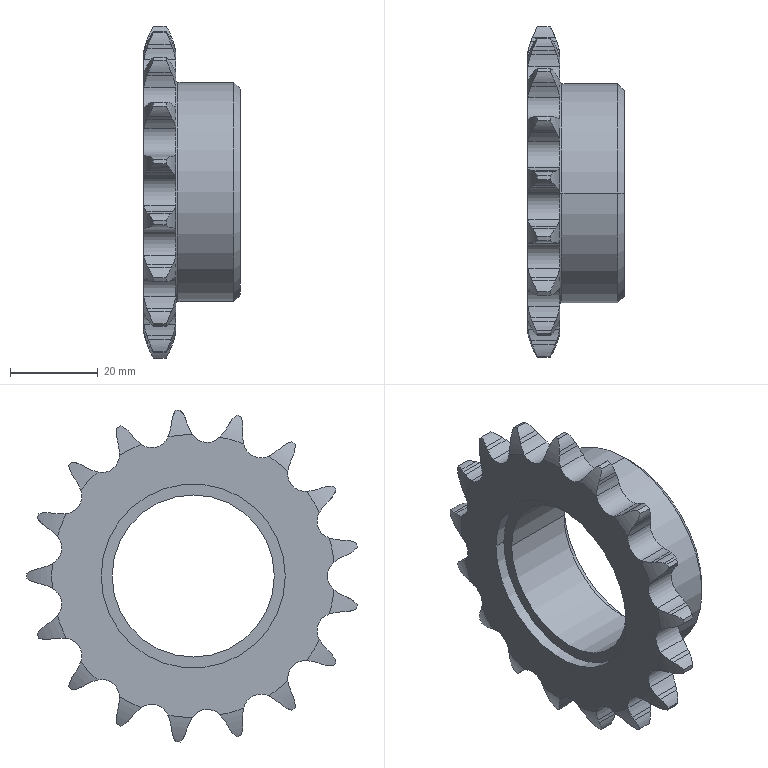Part | STEP file | J012-EBZ05-04-06-Part-1 | 1 solid | 195 faces | box 22 x 75.443 x 75.763 mm | volume 28418 mm3 | cylinder 118 | plane 39 | torus 36 | cone 2 | commonest cylinder face diameters 13.136 x36 20.708 x35 8.036 x22 76 x17 42 x4 37 x2